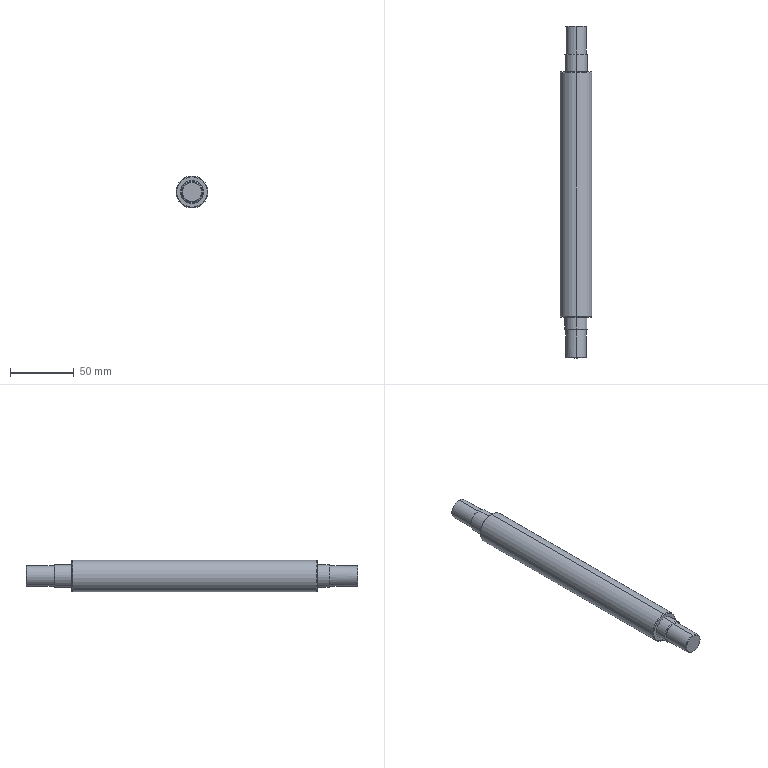Part | SolidWorks | features BaseBody 1 | 1 solid | 28 faces | box 25 x 260.5 x 25 mm | volume 109382 mm3 | cone 12 | cylinder 10 | plane 6 | commonest cylinder face diameters 16 x4 18 x4 25 x2
STEP:
#1=CARTESIAN_POINT('',(0.,32.6,12.5));
#2=VERTEX_POINT('',#1);
#3=CARTESIAN_POINT('',(0.,32.6,-12.5));
#4=VERTEX_POINT('',#3);
#5=CARTESIAN_POINT('',(0.,32.6,0.));
#6=DIRECTION('',(0.,1.,0.));
#7=DIRECTION('',(0.,0.,1.));
#8=AXIS2_PLACEMENT_3D('',#5,#6,#7);
#9=CIRCLE('',#8,12.5);
#10=EDGE_CURVE('',#2,#4,#9,.T.);
#11=ORIENTED_EDGE('',*,*,#10,.T.);
#12=CARTESIAN_POINT('',(0.,223.9,-12.5));
#13=VERTEX_POINT('',#12);
#14=CARTESIAN_POINT('',(0.,260.5,-12.5));
#15=DIRECTION('',(0.,1.,0.));
#16=VECTOR('',#15,1000.);
#17=LINE('',#14,#16);
#18=EDGE_CURVE('',#4,#13,#17,.T.);
#19=ORIENTED_EDGE('',*,*,#18,.T.);
#20=CARTESIAN_POINT('',(0.,223.9,12.5));
#21=VERTEX_POINT('',#20);
#22=CARTESIAN_POINT('',(0.,223.9,0.));
#23=DIRECTION('',(0.,-1.,0.));
#24=DIRECTION('',(0.,0.,1.));
#25=AXIS2_PLACEMENT_3D('',#22,#23,#24);
#26=CIRCLE('',#25,12.5);
#27=EDGE_CURVE('',#13,#21,#26,.T.);
#28=ORIENTED_EDGE('',*,*,#27,.T.);
#29=CARTESIAN_POINT('',(0.,260.5,12.5));
#30=DIRECTION('',(0.,1.,0.));
#31=VECTOR('',#30,1000.);
#32=LINE('',#29,#31);
#33=EDGE_CURVE('',#2,#21,#32,.T.);
#34=ORIENTED_EDGE('',*,*,#33,.F.);
#35=EDGE_LOOP('',(#11,#19,#28,#34));
#36=FACE_OUTER_BOUND('',#35,.T.);
#37=CARTESIAN_POINT('',(0.,260.5,0.));
#38=DIRECTION('',(0.,1.,0.));
#39=DIRECTION('',(0.,0.,1.));
#40=AXIS2_PLACEMENT_3D('',#37,#38,#39);
#41=CYLINDRICAL_SURFACE('',#40,12.5);
#42=ADVANCED_FACE('',(#36),#41,.T.);
#43=CARTESIAN_POINT('',(0.,224.5,-11.9));
#44=VERTEX_POINT('',#43);
#45=CARTESIAN_POINT('',(0.,224.5,11.9));
#46=VERTEX_POINT('',#45);
#47=CARTESIAN_POINT('',(0.,224.5,0.));
#48=DIRECTION('',(0.,-1.,0.));
#49=DIRECTION('',(0.,0.,-1.));
#50=AXIS2_PLACEMENT_3D('',#47,#48,#49);
#51=CIRCLE('',#50,11.9);
#52=EDGE_CURVE('',#44,#46,#51,.T.);
#53=ORIENTED_EDGE('',*,*,#52,.T.);
#54=CARTESIAN_POINT('',(0.,223.9,12.5));
#55=DIRECTION('',(0.,-0.7071,0.7071));
#56=VECTOR('',#55,1000.);
#57=LINE('',#54,#56);
#58=EDGE_CURVE('',#46,#21,#57,.T.);
#59=ORIENTED_EDGE('',*,*,#58,.T.);
#60=ORIENTED_EDGE('',*,*,#27,.F.);
#61=CARTESIAN_POINT('',(0.,223.9,-12.5));
#62=DIRECTION('',(0.,-0.7071,-0.7071));
#63=VECTOR('',#62,1000.);
#64=LINE('',#61,#63);
#65=EDGE_CURVE('',#44,#13,#64,.T.);
#66=ORIENTED_EDGE('',*,*,#65,.F.);
#67=EDGE_LOOP('',(#53,#59,#60,#66));
#68=FACE_OUTER_BOUND('',#67,.T.);
#69=CARTESIAN_POINT('',(0.,223.9,0.));
#70=DIRECTION('',(0.,-1.,0.));
#71=DIRECTION('',(0.,0.,-1.));
#72=AXIS2_PLACEMENT_3D('',#69,#70,#71);
#73=CONICAL_SURFACE('',#72,12.5,0.7854);
#74=ADVANCED_FACE('',(#68),#73,.T.);
#75=CARTESIAN_POINT('',(0.,32.,11.9));
#76=VERTEX_POINT('',#75);
#77=CARTESIAN_POINT('',(0.,32.,-11.9));
#78=VERTEX_POINT('',#77);
#79=CARTESIAN_POINT('',(0.,32.,0.));
#80=DIRECTION('',(0.,1.,0.));
#81=DIRECTION('',(0.,0.,1.));
#82=AXIS2_PLACEMENT_3D('',#79,#80,#81);
#83=CIRCLE('',#82,11.9);
#84=EDGE_CURVE('',#76,#78,#83,.T.);
#85=ORIENTED_EDGE('',*,*,#84,.T.);
#86=CARTESIAN_POINT('',(0.,32.6,-12.5));
#87=DIRECTION('',(0.,0.7071,-0.7071));
#88=VECTOR('',#87,1000.);
#89=LINE('',#86,#88);
#90=EDGE_CURVE('',#78,#4,#89,.T.);
#91=ORIENTED_EDGE('',*,*,#90,.T.);
#92=ORIENTED_EDGE('',*,*,#10,.F.);
#93=CARTESIAN_POINT('',(0.,32.6,12.5));
#94=DIRECTION('',(0.,0.7071,0.7071));
#95=VECTOR('',#94,1000.);
#96=LINE('',#93,#95);
#97=EDGE_CURVE('',#76,#2,#96,.T.);
#98=ORIENTED_EDGE('',*,*,#97,.F.);
#99=EDGE_LOOP('',(#85,#91,#92,#98));
#100=FACE_OUTER_BOUND('',#99,.T.);
#101=CARTESIAN_POINT('',(0.,32.6,0.));
#102=DIRECTION('',(0.,1.,0.));
#103=DIRECTION('',(0.,0.,1.));
#104=AXIS2_PLACEMENT_3D('',#101,#102,#103);
#105=CONICAL_SURFACE('',#104,12.5,0.7854);
#106=ADVANCED_FACE('',(#100),#105,.T.);
#107=CARTESIAN_POINT('',(0.,224.5,-9.));
#108=VERTEX_POINT('',#107);
#109=CARTESIAN_POINT('',(0.,224.5,9.));
#110=VERTEX_POINT('',#109);
#111=CARTESIAN_POINT('',(0.,224.5,0.));
#112=DIRECTION('',(0.,-1.,0.));
#113=DIRECTION('',(0.,0.,1.));
#114=AXIS2_PLACEMENT_3D('',#111,#112,#113);
#115=CIRCLE('',#114,9.);
#116=EDGE_CURVE('',#108,#110,#115,.T.);
#117=ORIENTED_EDGE('',*,*,#116,.F.);
#118=CARTESIAN_POINT('',(0.,237.9,-9.));
#119=VERTEX_POINT('',#118);
#120=CARTESIAN_POINT('',(0.,260.5,-9.));
#121=DIRECTION('',(0.,1.,0.));
#122=VECTOR('',#121,1000.);
#123=LINE('',#120,#122);
#124=EDGE_CURVE('',#108,#119,#123,.T.);
#125=ORIENTED_EDGE('',*,*,#124,.T.);
#126=CARTESIAN_POINT('',(0.,237.9,9.));
#127=VERTEX_POINT('',#126);
#128=CARTESIAN_POINT('',(0.,237.9,0.));
#129=DIRECTION('',(0.,-1.,0.));
#130=DIRECTION('',(0.,0.,1.));
#131=AXIS2_PLACEMENT_3D('',#128,#129,#130);
#132=CIRCLE('',#131,9.);
#133=EDGE_CURVE('',#119,#127,#132,.T.);
#134=ORIENTED_EDGE('',*,*,#133,.T.);
#135=CARTESIAN_POINT('',(0.,260.5,9.));
#136=DIRECTION('',(0.,1.,0.));
#137=VECTOR('',#136,1000.);
#138=LINE('',#135,#137);
#139=EDGE_CURVE('',#110,#127,#138,.T.);
#140=ORIENTED_EDGE('',*,*,#139,.F.);
#141=EDGE_LOOP('',(#117,#125,#134,#140));
#142=FACE_OUTER_BOUND('',#141,.T.);
#143=CARTESIAN_POINT('',(0.,260.5,0.));
#144=DIRECTION('',(0.,1.,0.));
#145=DIRECTION('',(0.,0.,1.));
#146=AXIS2_PLACEMENT_3D('',#143,#144,#145);
#147=CYLINDRICAL_SURFACE('',#146,9.);
#148=ADVANCED_FACE('',(#142),#147,.T.);
#149=CARTESIAN_POINT('',(0.,22.6,9.));
#150=VERTEX_POINT('',#149);
#151=CARTESIAN_POINT('',(0.,22.6,-9.));
#152=VERTEX_POINT('',#151);
#153=CARTESIAN_POINT('',(0.,22.6,0.));
#154=DIRECTION('',(0.,1.,0.));
#155=DIRECTION('',(0.,0.,1.));
#156=AXIS2_PLACEMENT_3D('',#153,#154,#155);
#157=CIRCLE('',#156,9.);
#158=EDGE_CURVE('',#150,#152,#157,.T.);
#159=ORIENTED_EDGE('',*,*,#158,.T.);
#160=CARTESIAN_POINT('',(0.,32.,-9.));
#161=VERTEX_POINT('',#160);
#162=CARTESIAN_POINT('',(0.,260.5,-9.));
#163=DIRECTION('',(0.,1.,0.));
#164=VECTOR('',#163,1000.);
#165=LINE('',#162,#164);
#166=EDGE_CURVE('',#152,#161,#165,.T.);
#167=ORIENTED_EDGE('',*,*,#166,.T.);
#168=CARTESIAN_POINT('',(0.,32.,9.));
#169=VERTEX_POINT('',#168);
#170=CARTESIAN_POINT('',(0.,32.,0.));
#171=DIRECTION('',(0.,1.,0.));
#172=DIRECTION('',(0.,0.,1.));
#173=AXIS2_PLACEMENT_3D('',#170,#171,#172);
#174=CIRCLE('',#173,9.);
#175=EDGE_CURVE('',#169,#161,#174,.T.);
#176=ORIENTED_EDGE('',*,*,#175,.F.);
#177=CARTESIAN_POINT('',(0.,260.5,9.));
#178=DIRECTION('',(0.,1.,0.));
#179=VECTOR('',#178,1000.);
#180=LINE('',#177,#179);
#181=EDGE_CURVE('',#150,#169,#180,.T.);
#182=ORIENTED_EDGE('',*,*,#181,.F.);
#183=EDGE_LOOP('',(#159,#167,#176,#182));
#184=FACE_OUTER_BOUND('',#183,.T.);
#185=CARTESIAN_POINT('',(0.,260.5,0.));
#186=DIRECTION('',(0.,1.,0.));
#187=DIRECTION('',(0.,0.,1.));
#188=AXIS2_PLACEMENT_3D('',#185,#186,#187);
#189=CYLINDRICAL_SURFACE('',#188,9.);
#190=ADVANCED_FACE('',(#184),#189,.T.);
#191=CARTESIAN_POINT('',(0.,238.5,-8.4));
#192=VERTEX_POINT('',#191);
#193=CARTESIAN_POINT('',(0.,238.5,8.4));
#194=VERTEX_POINT('',#193);
#195=CARTESIAN_POINT('',(0.,238.5,0.));
#196=DIRECTION('',(0.,-1.,0.));
#197=DIRECTION('',(0.,0.,-1.));
#198=AXIS2_PLACEMENT_3D('',#195,#196,#197);
#199=CIRCLE('',#198,8.4);
#200=EDGE_CURVE('',#192,#194,#199,.T.);
#201=ORIENTED_EDGE('',*,*,#200,.T.);
#202=CARTESIAN_POINT('',(0.,237.9,9.));
#203=DIRECTION('',(0.,-0.7071,0.7071));
#204=VECTOR('',#203,1000.);
#205=LINE('',#202,#204);
#206=EDGE_CURVE('',#194,#127,#205,.T.);
#207=ORIENTED_EDGE('',*,*,#206,.T.);
#208=ORIENTED_EDGE('',*,*,#133,.F.);
#209=CARTESIAN_POINT('',(0.,237.9,-9.));
#210=DIRECTION('',(0.,-0.7071,-0.7071));
#211=VECTOR('',#210,1000.);
#212=LINE('',#209,#211);
#213=EDGE_CURVE('',#192,#119,#212,.T.);
#214=ORIENTED_EDGE('',*,*,#213,.F.);
#215=EDGE_LOOP('',(#201,#207,#208,#214));
#216=FACE_OUTER_BOUND('',#215,.T.);
#217=CARTESIAN_POINT('',(0.,237.9,0.));
#218=DIRECTION('',(0.,-1.,0.));
#219=DIRECTION('',(0.,0.,-1.));
#220=AXIS2_PLACEMENT_3D('',#217,#218,#219);
#221=CONICAL_SURFACE('',#220,9.,0.7854);
#222=ADVANCED_FACE('',(#216),#221,.T.);
#223=CARTESIAN_POINT('',(0.,22.,8.4));
#224=VERTEX_POINT('',#223);
#225=CARTESIAN_POINT('',(0.,22.,-8.4));
#226=VERTEX_POINT('',#225);
#227=CARTESIAN_POINT('',(0.,22.,0.));
#228=DIRECTION('',(0.,1.,0.));
#229=DIRECTION('',(0.,0.,1.));
#230=AXIS2_PLACEMENT_3D('',#227,#228,#229);
#231=CIRCLE('',#230,8.4);
#232=EDGE_CURVE('',#224,#226,#231,.T.);
#233=ORIENTED_EDGE('',*,*,#232,.T.);
#234=CARTESIAN_POINT('',(0.,22.6,-9.));
#235=DIRECTION('',(0.,0.7071,-0.7071));
#236=VECTOR('',#235,1000.);
#237=LINE('',#234,#236);
#238=EDGE_CURVE('',#226,#152,#237,.T.);
#239=ORIENTED_EDGE('',*,*,#238,.T.);
#240=ORIENTED_EDGE('',*,*,#158,.F.);
#241=CARTESIAN_POINT('',(0.,22.6,9.));
#242=DIRECTION('',(0.,0.7071,0.7071));
#243=VECTOR('',#242,1000.);
#244=LINE('',#241,#243);
#245=EDGE_CURVE('',#224,#150,#244,.T.);
#246=ORIENTED_EDGE('',*,*,#245,.F.);
#247=EDGE_LOOP('',(#233,#239,#240,#246));
#248=FACE_OUTER_BOUND('',#247,.T.);
#249=CARTESIAN_POINT('',(0.,22.6,0.));
#250=DIRECTION('',(0.,1.,0.));
#251=DIRECTION('',(0.,0.,1.));
#252=AXIS2_PLACEMENT_3D('',#249,#250,#251);
#253=CONICAL_SURFACE('',#252,9.,0.7854);
#254=ADVANCED_FACE('',(#248),#253,.T.);
#255=CARTESIAN_POINT('',(0.,238.5,-8.));
#256=VERTEX_POINT('',#255);
#257=CARTESIAN_POINT('',(0.,238.5,8.));
#258=VERTEX_POINT('',#257);
#259=CARTESIAN_POINT('',(0.,238.5,0.));
#260=DIRECTION('',(0.,-1.,0.));
#261=DIRECTION('',(0.,0.,1.));
#262=AXIS2_PLACEMENT_3D('',#259,#260,#261);
#263=CIRCLE('',#262,8.);
#264=EDGE_CURVE('',#256,#258,#263,.T.);
#265=ORIENTED_EDGE('',*,*,#264,.F.);
#266=CARTESIAN_POINT('',(0.,259.9,-8.));
#267=VERTEX_POINT('',#266);
#268=CARTESIAN_POINT('',(0.,260.5,-8.));
#269=DIRECTION('',(0.,1.,0.));
#270=VECTOR('',#269,1000.);
#271=LINE('',#268,#270);
#272=EDGE_CURVE('',#256,#267,#271,.T.);
#273=ORIENTED_EDGE('',*,*,#272,.T.);
#274=CARTESIAN_POINT('',(0.,259.9,8.));
#275=VERTEX_POINT('',#274);
#276=CARTESIAN_POINT('',(0.,259.9,0.));
#277=DIRECTION('',(0.,-1.,0.));
#278=DIRECTION('',(0.,0.,1.));
#279=AXIS2_PLACEMENT_3D('',#276,#277,#278);
#280=CIRCLE('',#279,8.);
#281=EDGE_CURVE('',#267,#275,#280,.T.);
#282=ORIENTED_EDGE('',*,*,#281,.T.);
#283=CARTESIAN_POINT('',(0.,260.5,8.));
#284=DIRECTION('',(0.,1.,0.));
#285=VECTOR('',#284,1000.);
#286=LINE('',#283,#285);
#287=EDGE_CURVE('',#258,#275,#286,.T.);
#288=ORIENTED_EDGE('',*,*,#287,.F.);
#289=EDGE_LOOP('',(#265,#273,#282,#288));
#290=FACE_OUTER_BOUND('',#289,.T.);
#291=CARTESIAN_POINT('',(0.,260.5,0.));
#292=DIRECTION('',(0.,1.,0.));
#293=DIRECTION('',(0.,0.,1.));
#294=AXIS2_PLACEMENT_3D('',#291,#292,#293);
#295=CYLINDRICAL_SURFACE('',#294,8.);
#296=ADVANCED_FACE('',(#290),#295,.T.);
#297=CARTESIAN_POINT('',(8.,0.6,0.));
#298=VERTEX_POINT('',#297);
#299=CARTESIAN_POINT('',(0.,0.6,-8.));
#300=VERTEX_POINT('',#299);
#301=CARTESIAN_POINT('',(0.,0.6,0.));
#302=DIRECTION('',(0.,1.,0.));
#303=DIRECTION('',(0.,0.,1.));
#304=AXIS2_PLACEMENT_3D('',#301,#302,#303);
#305=CIRCLE('',#304,8.);
#306=EDGE_CURVE('',#298,#300,#305,.T.);
#307=ORIENTED_EDGE('',*,*,#306,.T.);
#308=CARTESIAN_POINT('',(0.,22.,-8.));
#309=VERTEX_POINT('',#308);
#310=CARTESIAN_POINT('',(0.,260.5,-8.));
#311=DIRECTION('',(0.,1.,0.));
#312=VECTOR('',#311,1000.);
#313=LINE('',#310,#312);
#314=EDGE_CURVE('',#300,#309,#313,.T.);
#315=ORIENTED_EDGE('',*,*,#314,.T.);
#316=CARTESIAN_POINT('',(0.,22.,8.));
#317=VERTEX_POINT('',#316);
#318=CARTESIAN_POINT('',(0.,22.,0.));
#319=DIRECTION('',(0.,1.,0.));
#320=DIRECTION('',(0.,0.,1.));
#321=AXIS2_PLACEMENT_3D('',#318,#319,#320);
#322=CIRCLE('',#321,8.);
#323=EDGE_CURVE('',#317,#309,#322,.T.);
#324=ORIENTED_EDGE('',*,*,#323,.F.);
#325=CARTESIAN_POINT('',(0.,0.6,8.));
#326=VERTEX_POINT('',#325);
#327=CARTESIAN_POINT('',(0.,260.5,8.));
#328=DIRECTION('',(0.,1.,0.));
#329=VECTOR('',#328,1000.);
#330=LINE('',#327,#329);
#331=EDGE_CURVE('',#326,#317,#330,.T.);
#332=ORIENTED_EDGE('',*,*,#331,.F.);
#333=CARTESIAN_POINT('',(0.,0.6,0.));
#334=DIRECTION('',(0.,1.,0.));
#335=DIRECTION('',(0.,0.,1.));
#336=AXIS2_PLACEMENT_3D('',#333,#334,#335);
#337=CIRCLE('',#336,8.);
#338=EDGE_CURVE('',#326,#298,#337,.T.);
#339=ORIENTED_EDGE('',*,*,#338,.T.);
#340=EDGE_LOOP('',(#307,#315,#324,#332,#339));
#341=FACE_OUTER_BOUND('',#340,.T.);
#342=CARTESIAN_POINT('',(0.,260.5,0.));
#343=DIRECTION('',(0.,1.,0.));
#344=DIRECTION('',(0.,0.,1.));
#345=AXIS2_PLACEMENT_3D('',#342,#343,#344);
#346=CYLINDRICAL_SURFACE('',#345,8.);
#347=ADVANCED_FACE('',(#341),#346,.T.);
#348=CARTESIAN_POINT('',(0.,260.5,-7.4));
#349=VERTEX_POINT('',#348);
#350=CARTESIAN_POINT('',(0.,260.5,7.4));
#351=VERTEX_POINT('',#350);
#352=CARTESIAN_POINT('',(0.,260.5,0.));
#353=DIRECTION('',(0.,-1.,0.));
#354=DIRECTION('',(0.,0.,-1.));
#355=AXIS2_PLACEMENT_3D('',#352,#353,#354);
#356=CIRCLE('',#355,7.4);
#357=EDGE_CURVE('',#349,#351,#356,.T.);
#358=ORIENTED_EDGE('',*,*,#357,.T.);
#359=CARTESIAN_POINT('',(0.,259.9,8.));
#360=DIRECTION('',(0.,-0.7071,0.7071));
#361=VECTOR('',#360,1000.);
#362=LINE('',#359,#361);
#363=EDGE_CURVE('',#351,#275,#362,.T.);
#364=ORIENTED_EDGE('',*,*,#363,.T.);
#365=ORIENTED_EDGE('',*,*,#281,.F.);
#366=CARTESIAN_POINT('',(0.,259.9,-8.));
#367=DIRECTION('',(0.,-0.7071,-0.7071));
#368=VECTOR('',#367,1000.);
#369=LINE('',#366,#368);
#370=EDGE_CURVE('',#349,#267,#369,.T.);
#371=ORIENTED_EDGE('',*,*,#370,.F.);
#372=EDGE_LOOP('',(#358,#364,#365,#371));
#373=FACE_OUTER_BOUND('',#372,.T.);
#374=CARTESIAN_POINT('',(0.,259.9,0.));
#375=DIRECTION('',(0.,-1.,0.));
#376=DIRECTION('',(0.,0.,-1.));
#377=AXIS2_PLACEMENT_3D('',#374,#375,#376);
#378=CONICAL_SURFACE('',#377,8.,0.7854);
#379=ADVANCED_FACE('',(#373),#378,.T.);
#380=CARTESIAN_POINT('',(-7.4,0.,0.));
#381=VERTEX_POINT('',#380);
#382=CARTESIAN_POINT('',(7.4,0.,0.));
#383=VERTEX_POINT('',#382);
#384=CARTESIAN_POINT('',(0.,0.,0.));
#385=DIRECTION('',(0.,1.,0.));
#386=DIRECTION('',(-1.,0.,0.));
#387=AXIS2_PLACEMENT_3D('',#384,#385,#386);
#388=CIRCLE('',#387,7.4);
#389=EDGE_CURVE('',#381,#383,#388,.T.);
#390=ORIENTED_EDGE('',*,*,#389,.T.);
#391=CARTESIAN_POINT('',(8.,0.6,0.));
#392=DIRECTION('',(0.7071,0.7071,0.));
#393=VECTOR('',#392,1000.);
#394=LINE('',#391,#393);
#395=EDGE_CURVE('',#383,#298,#394,.T.);
#396=ORIENTED_EDGE('',*,*,#395,.T.);
#397=ORIENTED_EDGE('',*,*,#338,.F.);
#398=CARTESIAN_POINT('',(-8.,0.6,0.));
#399=VERTEX_POINT('',#398);
#400=CARTESIAN_POINT('',(0.,0.6,0.));
#401=DIRECTION('',(0.,1.,0.));
#402=DIRECTION('',(0.,0.,1.));
#403=AXIS2_PLACEMENT_3D('',#400,#401,#402);
#404=CIRCLE('',#403,8.);
#405=EDGE_CURVE('',#399,#326,#404,.T.);
#406=ORIENTED_EDGE('',*,*,#405,.F.);
#407=CARTESIAN_POINT('',(-8.,0.6,0.));
#408=DIRECTION('',(-0.7071,0.7071,0.));
#409=VECTOR('',#408,1000.);
#410=LINE('',#407,#409);
#411=EDGE_CURVE('',#381,#399,#410,.T.);
#412=ORIENTED_EDGE('',*,*,#411,.F.);
#413=EDGE_LOOP('',(#390,#396,#397,#406,#412));
#414=FACE_OUTER_BOUND('',#413,.T.);
#415=CARTESIAN_POINT('',(0.,0.6,0.));
#416=DIRECTION('',(0.,1.,0.));
#417=DIRECTION('',(-1.,0.,0.));
#418=AXIS2_PLACEMENT_3D('',#415,#416,#417);
#419=CONICAL_SURFACE('',#418,8.,0.7854);
#420=ADVANCED_FACE('',(#414),#419,.T.);
#421=ORIENTED_EDGE('',*,*,#18,.F.);
#422=CARTESIAN_POINT('',(0.,32.6,0.));
#423=DIRECTION('',(0.,1.,0.));
#424=DIRECTION('',(0.,0.,1.));
#425=AXIS2_PLACEMENT_3D('',#422,#423,#424);
#426=CIRCLE('',#425,12.5);
#427=EDGE_CURVE('',#4,#2,#426,.T.);
#428=ORIENTED_EDGE('',*,*,#427,.T.);
#429=ORIENTED_EDGE('',*,*,#33,.T.);
#430=CARTESIAN_POINT('',(0.,223.9,0.));
#431=DIRECTION('',(0.,-1.,0.));
#432=DIRECTION('',(0.,0.,1.));
#433=AXIS2_PLACEMENT_3D('',#430,#431,#432);
#434=CIRCLE('',#433,12.5);
#435=EDGE_CURVE('',#21,#13,#434,.T.);
#436=ORIENTED_EDGE('',*,*,#435,.T.);
#437=EDGE_LOOP('',(#421,#428,#429,#436));
#438=FACE_OUTER_BOUND('',#437,.T.);
#439=CARTESIAN_POINT('',(0.,260.5,0.));
#440=DIRECTION('',(0.,1.,0.));
#441=DIRECTION('',(0.,0.,1.));
#442=AXIS2_PLACEMENT_3D('',#439,#440,#441);
#443=CYLINDRICAL_SURFACE('',#442,12.5);
#444=ADVANCED_FACE('',(#438),#443,.T.);
#445=ORIENTED_EDGE('',*,*,#58,.F.);
#446=CARTESIAN_POINT('',(0.,224.5,0.));
#447=DIRECTION('',(0.,-1.,0.));
#448=DIRECTION('',(0.,0.,-1.));
#449=AXIS2_PLACEMENT_3D('',#446,#447,#448);
#450=CIRCLE('',#449,11.9);
#451=EDGE_CURVE('',#46,#44,#450,.T.);
#452=ORIENTED_EDGE('',*,*,#451,.T.);
#453=ORIENTED_EDGE('',*,*,#65,.T.);
#454=ORIENTED_EDGE('',*,*,#435,.F.);
#455=EDGE_LOOP('',(#445,#452,#453,#454));
#456=FACE_OUTER_BOUND('',#455,.T.);
#457=CARTESIAN_POINT('',(0.,223.9,0.));
#458=DIRECTION('',(0.,-1.,0.));
#459=DIRECTION('',(0.,0.,-1.));
#460=AXIS2_PLACEMENT_3D('',#457,#458,#459);
#461=CONICAL_SURFACE('',#460,12.5,0.7854);
#462=ADVANCED_FACE('',(#456),#461,.T.);
#463=ORIENTED_EDGE('',*,*,#90,.F.);
#464=CARTESIAN_POINT('',(0.,32.,0.));
#465=DIRECTION('',(0.,1.,0.));
#466=DIRECTION('',(0.,0.,1.));
#467=AXIS2_PLACEMENT_3D('',#464,#465,#466);
#468=CIRCLE('',#467,11.9);
#469=EDGE_CURVE('',#78,#76,#468,.T.);
#470=ORIENTED_EDGE('',*,*,#469,.T.);
#471=ORIENTED_EDGE('',*,*,#97,.T.);
#472=ORIENTED_EDGE('',*,*,#427,.F.);
#473=EDGE_LOOP('',(#463,#470,#471,#472));
#474=FACE_OUTER_BOUND('',#473,.T.);
#475=CARTESIAN_POINT('',(0.,32.6,0.));
#476=DIRECTION('',(0.,1.,0.));
#477=DIRECTION('',(0.,0.,1.));
#478=AXIS2_PLACEMENT_3D('',#475,#476,#477);
#479=CONICAL_SURFACE('',#478,12.5,0.7854);
#480=ADVANCED_FACE('',(#474),#479,.T.);
#481=CARTESIAN_POINT('',(0.,224.5,0.));
#482=DIRECTION('',(0.,-1.,0.));
#483=DIRECTION('',(0.,0.,1.));
#484=AXIS2_PLACEMENT_3D('',#481,#482,#483);
#485=CIRCLE('',#484,9.);
#486=EDGE_CURVE('',#110,#108,#485,.T.);
#487=ORIENTED_EDGE('',*,*,#486,.T.);
#488=ORIENTED_EDGE('',*,*,#116,.T.);
#489=EDGE_LOOP('',(#487,#488));
#490=FACE_BOUND('',#489,.T.);
#491=ORIENTED_EDGE('',*,*,#52,.F.);
#492=ORIENTED_EDGE('',*,*,#451,.F.);
#493=EDGE_LOOP('',(#491,#492));
#494=FACE_OUTER_BOUND('',#493,.T.);
#495=CARTESIAN_POINT('',(-11.9,224.5,0.));
#496=DIRECTION('',(0.,1.,0.));
#497=DIRECTION('',(-1.,0.,0.));
#498=AXIS2_PLACEMENT_3D('',#495,#496,#497);
#499=PLANE('',#498);
#500=ADVANCED_FACE('',(#490,#494),#499,.T.);
#501=ORIENTED_EDGE('',*,*,#175,.T.);
#502=CARTESIAN_POINT('',(0.,32.,0.));
#503=DIRECTION('',(0.,1.,0.));
#504=DIRECTION('',(0.,0.,1.));
#505=AXIS2_PLACEMENT_3D('',#502,#503,#504);
#506=CIRCLE('',#505,9.);
#507=EDGE_CURVE('',#161,#169,#506,.T.);
#508=ORIENTED_EDGE('',*,*,#507,.T.);
#509=EDGE_LOOP('',(#501,#508));
#510=FACE_BOUND('',#509,.T.);
#511=ORIENTED_EDGE('',*,*,#84,.F.);
#512=ORIENTED_EDGE('',*,*,#469,.F.);
#513=EDGE_LOOP('',(#511,#512));
#514=FACE_OUTER_BOUND('',#513,.T.);
#515=CARTESIAN_POINT('',(-9.,32.,0.));
#516=DIRECTION('',(0.,-1.,0.));
#517=DIRECTION('',(1.,0.,0.));
#518=AXIS2_PLACEMENT_3D('',#515,#516,#517);
#519=PLANE('',#518);
#520=ADVANCED_FACE('',(#510,#514),#519,.T.);
#521=ORIENTED_EDGE('',*,*,#124,.F.);
#522=ORIENTED_EDGE('',*,*,#486,.F.);
#523=ORIENTED_EDGE('',*,*,#139,.T.);
#524=CARTESIAN_POINT('',(0.,237.9,0.));
#525=DIRECTION('',(0.,-1.,0.));
#526=DIRECTION('',(0.,0.,1.));
#527=AXIS2_PLACEMENT_3D('',#524,#525,#526);
#528=CIRCLE('',#527,9.);
#529=EDGE_CURVE('',#127,#119,#528,.T.);
#530=ORIENTED_EDGE('',*,*,#529,.T.);
#531=EDGE_LOOP('',(#521,#522,#523,#530));
#532=FACE_OUTER_BOUND('',#531,.T.);
#533=CARTESIAN_POINT('',(0.,260.5,0.));
#534=DIRECTION('',(0.,1.,0.));
#535=DIRECTION('',(0.,0.,1.));
#536=AXIS2_PLACEMENT_3D('',#533,#534,#535);
#537=CYLINDRICAL_SURFACE('',#536,9.);
#538=ADVANCED_FACE('',(#532),#537,.T.);
#539=ORIENTED_EDGE('',*,*,#166,.F.);
#540=CARTESIAN_POINT('',(0.,22.6,0.));
#541=DIRECTION('',(0.,1.,0.));
#542=DIRECTION('',(0.,0.,1.));
#543=AXIS2_PLACEMENT_3D('',#540,#541,#542);
#544=CIRCLE('',#543,9.);
#545=EDGE_CURVE('',#152,#150,#544,.T.);
#546=ORIENTED_EDGE('',*,*,#545,.T.);
#547=ORIENTED_EDGE('',*,*,#181,.T.);
#548=ORIENTED_EDGE('',*,*,#507,.F.);
#549=EDGE_LOOP('',(#539,#546,#547,#548));
#550=FACE_OUTER_BOUND('',#549,.T.);
#551=CARTESIAN_POINT('',(0.,260.5,0.));
#552=DIRECTION('',(0.,1.,0.));
#553=DIRECTION('',(0.,0.,1.));
#554=AXIS2_PLACEMENT_3D('',#551,#552,#553);
#555=CYLINDRICAL_SURFACE('',#554,9.);
#556=ADVANCED_FACE('',(#550),#555,.T.);
#557=ORIENTED_EDGE('',*,*,#206,.F.);
#558=CARTESIAN_POINT('',(0.,238.5,0.));
#559=DIRECTION('',(0.,-1.,0.));
#560=DIRECTION('',(0.,0.,-1.));
#561=AXIS2_PLACEMENT_3D('',#558,#559,#560);
#562=CIRCLE('',#561,8.4);
#563=EDGE_CURVE('',#194,#192,#562,.T.);
#564=ORIENTED_EDGE('',*,*,#563,.T.);
#565=ORIENTED_EDGE('',*,*,#213,.T.);
#566=ORIENTED_EDGE('',*,*,#529,.F.);
#567=EDGE_LOOP('',(#557,#564,#565,#566));
#568=FACE_OUTER_BOUND('',#567,.T.);
#569=CARTESIAN_POINT('',(0.,237.9,0.));
#570=DIRECTION('',(0.,-1.,0.));
#571=DIRECTION('',(0.,0.,-1.));
#572=AXIS2_PLACEMENT_3D('',#569,#570,#571);
#573=CONICAL_SURFACE('',#572,9.,0.7854);
#574=ADVANCED_FACE('',(#568),#573,.T.);
#575=ORIENTED_EDGE('',*,*,#238,.F.);
#576=CARTESIAN_POINT('',(0.,22.,0.));
#577=DIRECTION('',(0.,1.,0.));
#578=DIRECTION('',(0.,0.,1.));
#579=AXIS2_PLACEMENT_3D('',#576,#577,#578);
#580=CIRCLE('',#579,8.4);
#581=EDGE_CURVE('',#226,#224,#580,.T.);
#582=ORIENTED_EDGE('',*,*,#581,.T.);
#583=ORIENTED_EDGE('',*,*,#245,.T.);
#584=ORIENTED_EDGE('',*,*,#545,.F.);
#585=EDGE_LOOP('',(#575,#582,#583,#584));
#586=FACE_OUTER_BOUND('',#585,.T.);
#587=CARTESIAN_POINT('',(0.,22.6,0.));
#588=DIRECTION('',(0.,1.,0.));
#589=DIRECTION('',(0.,0.,1.));
#590=AXIS2_PLACEMENT_3D('',#587,#588,#589);
#591=CONICAL_SURFACE('',#590,9.,0.7854);
#592=ADVANCED_FACE('',(#586),#591,.T.);
#593=CARTESIAN_POINT('',(0.,238.5,0.));
#594=DIRECTION('',(0.,-1.,0.));
#595=DIRECTION('',(0.,0.,1.));
#596=AXIS2_PLACEMENT_3D('',#593,#594,#595);
#597=CIRCLE('',#596,8.);
#598=EDGE_CURVE('',#258,#256,#597,.T.);
#599=ORIENTED_EDGE('',*,*,#598,.T.);
#600=ORIENTED_EDGE('',*,*,#264,.T.);
#601=EDGE_LOOP('',(#599,#600));
#602=FACE_BOUND('',#601,.T.);
#603=ORIENTED_EDGE('',*,*,#200,.F.);
#604=ORIENTED_EDGE('',*,*,#563,.F.);
#605=EDGE_LOOP('',(#603,#604));
#606=FACE_OUTER_BOUND('',#605,.T.);
#607=CARTESIAN_POINT('',(-8.4,238.5,0.));
#608=DIRECTION('',(0.,1.,0.));
#609=DIRECTION('',(-1.,0.,0.));
#610=AXIS2_PLACEMENT_3D('',#607,#608,#609);
#611=PLANE('',#610);
#612=ADVANCED_FACE('',(#602,#606),#611,.T.);
#613=ORIENTED_EDGE('',*,*,#323,.T.);
#614=CARTESIAN_POINT('',(0.,22.,0.));
#615=DIRECTION('',(0.,1.,0.));
#616=DIRECTION('',(0.,0.,1.));
#617=AXIS2_PLACEMENT_3D('',#614,#615,#616);
#618=CIRCLE('',#617,8.);
#619=EDGE_CURVE('',#309,#317,#618,.T.);
#620=ORIENTED_EDGE('',*,*,#619,.T.);
#621=EDGE_LOOP('',(#613,#620));
#622=FACE_BOUND('',#621,.T.);
#623=ORIENTED_EDGE('',*,*,#232,.F.);
#624=ORIENTED_EDGE('',*,*,#581,.F.);
#625=EDGE_LOOP('',(#623,#624));
#626=FACE_OUTER_BOUND('',#625,.T.);
#627=CARTESIAN_POINT('',(-8.,22.,0.));
#628=DIRECTION('',(0.,-1.,0.));
#629=DIRECTION('',(1.,0.,0.));
#630=AXIS2_PLACEMENT_3D('',#627,#628,#629);
#631=PLANE('',#630);
#632=ADVANCED_FACE('',(#622,#626),#631,.T.);
#633=ORIENTED_EDGE('',*,*,#272,.F.);
#634=ORIENTED_EDGE('',*,*,#598,.F.);
#635=ORIENTED_EDGE('',*,*,#287,.T.);
#636=CARTESIAN_POINT('',(0.,259.9,0.));
#637=DIRECTION('',(0.,-1.,0.));
#638=DIRECTION('',(0.,0.,1.));
#639=AXIS2_PLACEMENT_3D('',#636,#637,#638);
#640=CIRCLE('',#639,8.);
#641=EDGE_CURVE('',#275,#267,#640,.T.);
#642=ORIENTED_EDGE('',*,*,#641,.T.);
#643=EDGE_LOOP('',(#633,#634,#635,#642));
#644=FACE_OUTER_BOUND('',#643,.T.);
#645=CARTESIAN_POINT('',(0.,260.5,0.));
#646=DIRECTION('',(0.,1.,0.));
#647=DIRECTION('',(0.,0.,1.));
#648=AXIS2_PLACEMENT_3D('',#645,#646,#647);
#649=CYLINDRICAL_SURFACE('',#648,8.);
#650=ADVANCED_FACE('',(#644),#649,.T.);
#651=ORIENTED_EDGE('',*,*,#314,.F.);
#652=CARTESIAN_POINT('',(0.,0.6,0.));
#653=DIRECTION('',(0.,1.,0.));
#654=DIRECTION('',(0.,0.,1.));
#655=AXIS2_PLACEMENT_3D('',#652,#653,#654);
#656=CIRCLE('',#655,8.);
#657=EDGE_CURVE('',#300,#399,#656,.T.);
#658=ORIENTED_EDGE('',*,*,#657,.T.);
#659=ORIENTED_EDGE('',*,*,#405,.T.);
#660=ORIENTED_EDGE('',*,*,#331,.T.);
#661=ORIENTED_EDGE('',*,*,#619,.F.);
#662=EDGE_LOOP('',(#651,#658,#659,#660,#661));
#663=FACE_OUTER_BOUND('',#662,.T.);
#664=CARTESIAN_POINT('',(0.,260.5,0.));
#665=DIRECTION('',(0.,1.,0.));
#666=DIRECTION('',(0.,0.,1.));
#667=AXIS2_PLACEMENT_3D('',#664,#665,#666);
#668=CYLINDRICAL_SURFACE('',#667,8.);
#669=ADVANCED_FACE('',(#663),#668,.T.);
#670=ORIENTED_EDGE('',*,*,#363,.F.);
#671=CARTESIAN_POINT('',(0.,260.5,0.));
#672=DIRECTION('',(0.,-1.,0.));
#673=DIRECTION('',(0.,0.,-1.));
#674=AXIS2_PLACEMENT_3D('',#671,#672,#673);
#675=CIRCLE('',#674,7.4);
#676=EDGE_CURVE('',#351,#349,#675,.T.);
#677=ORIENTED_EDGE('',*,*,#676,.T.);
#678=ORIENTED_EDGE('',*,*,#370,.T.);
#679=ORIENTED_EDGE('',*,*,#641,.F.);
#680=EDGE_LOOP('',(#670,#677,#678,#679));
#681=FACE_OUTER_BOUND('',#680,.T.);
#682=CARTESIAN_POINT('',(0.,259.9,0.));
#683=DIRECTION('',(0.,-1.,0.));
#684=DIRECTION('',(0.,0.,-1.));
#685=AXIS2_PLACEMENT_3D('',#682,#683,#684);
#686=CONICAL_SURFACE('',#685,8.,0.7854);
#687=ADVANCED_FACE('',(#681),#686,.T.);
#688=ORIENTED_EDGE('',*,*,#395,.F.);
#689=CARTESIAN_POINT('',(0.,0.,0.));
#690=DIRECTION('',(0.,1.,0.));
#691=DIRECTION('',(-1.,0.,0.));
#692=AXIS2_PLACEMENT_3D('',#689,#690,#691);
#693=CIRCLE('',#692,7.4);
#694=EDGE_CURVE('',#383,#381,#693,.T.);
#695=ORIENTED_EDGE('',*,*,#694,.T.);
#696=ORIENTED_EDGE('',*,*,#411,.T.);
#697=ORIENTED_EDGE('',*,*,#657,.F.);
#698=ORIENTED_EDGE('',*,*,#306,.F.);
#699=EDGE_LOOP('',(#688,#695,#696,#697,#698));
#700=FACE_OUTER_BOUND('',#699,.T.);
#701=CARTESIAN_POINT('',(0.,0.6,0.));
#702=DIRECTION('',(0.,1.,0.));
#703=DIRECTION('',(-1.,0.,0.));
#704=AXIS2_PLACEMENT_3D('',#701,#702,#703);
#705=CONICAL_SURFACE('',#704,8.,0.7854);
#706=ADVANCED_FACE('',(#700),#705,.T.);
#707=ORIENTED_EDGE('',*,*,#357,.F.);
#708=ORIENTED_EDGE('',*,*,#676,.F.);
#709=EDGE_LOOP('',(#707,#708));
#710=FACE_OUTER_BOUND('',#709,.T.);
#711=CARTESIAN_POINT('',(-7.4,260.5,0.));
#712=DIRECTION('',(0.,1.,0.));
#713=DIRECTION('',(-1.,0.,0.));
#714=AXIS2_PLACEMENT_3D('',#711,#712,#713);
#715=PLANE('',#714);
#716=ADVANCED_FACE('',(#710),#715,.T.);
#717=ORIENTED_EDGE('',*,*,#389,.F.);
#718=ORIENTED_EDGE('',*,*,#694,.F.);
#719=EDGE_LOOP('',(#717,#718));
#720=FACE_OUTER_BOUND('',#719,.T.);
#721=CARTESIAN_POINT('',(0.,0.,0.));
#722=DIRECTION('',(0.,-1.,0.));
#723=DIRECTION('',(1.,0.,0.));
#724=AXIS2_PLACEMENT_3D('',#721,#722,#723);
#725=PLANE('',#724);
#726=ADVANCED_FACE('',(#720),#725,.T.);
#727=CLOSED_SHELL('',(#42,#74,#106,#148,#190,#222,#254,#296,#347,#379,#420,#444,#462,#480,#500,#520,#538,#556,#574,#592,#612,#632,#650,#669,#687,#706,#716,#726));
#728=MANIFOLD_SOLID_BREP('',#727);
#729=CARTESIAN_POINT('',(0.,0.,0.));
#730=DIRECTION('',(0.,0.,1.));
#731=DIRECTION('',(1.,0.,0.));
#732=AXIS2_PLACEMENT_3D('',#729,#730,#731);
#733=(LENGTH_UNIT()NAMED_UNIT(*)SI_UNIT(.MILLI.,.METRE.));
#734=UNCERTAINTY_MEASURE_WITH_UNIT(LENGTH_MEASURE(0.00001),#733,'','');
#735=(NAMED_UNIT(*)PLANE_ANGLE_UNIT()SI_UNIT($,.RADIAN.));
#736=(NAMED_UNIT(*)SI_UNIT($,.STERADIAN.)SOLID_ANGLE_UNIT());
#737=(GEOMETRIC_REPRESENTATION_CONTEXT(3)GLOBAL_UNCERTAINTY_ASSIGNED_CONTEXT((#734))GLOBAL_UNIT_ASSIGNED_CONTEXT((#733,#735,#736))REPRESENTATION_CONTEXT('',''));
#738=ADVANCED_BREP_SHAPE_REPRESENTATION('',(#728,#732),#737);